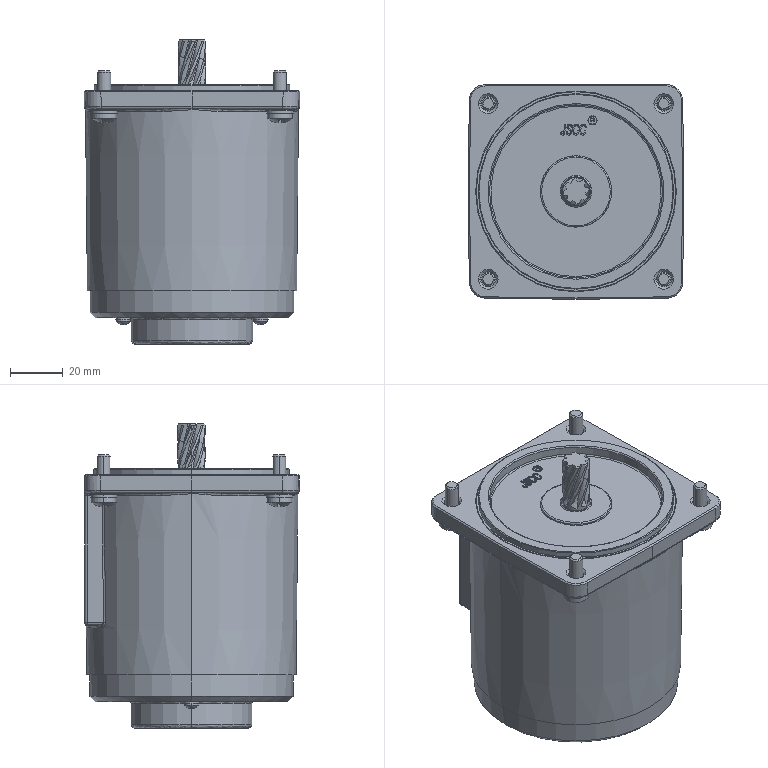Part | STEP file | 80YT25G | 1 solid | 665 faces | box 81.679 x 81.24 x 115.2 mm | volume 124196 mm3 | plane 260 | spline 230 | cylinder 132 | cone 39 | other 4 | commonest cylinder face diameters 1 x16 2 x15 3 x8 5 x8 5.8 x8 9.5 x8